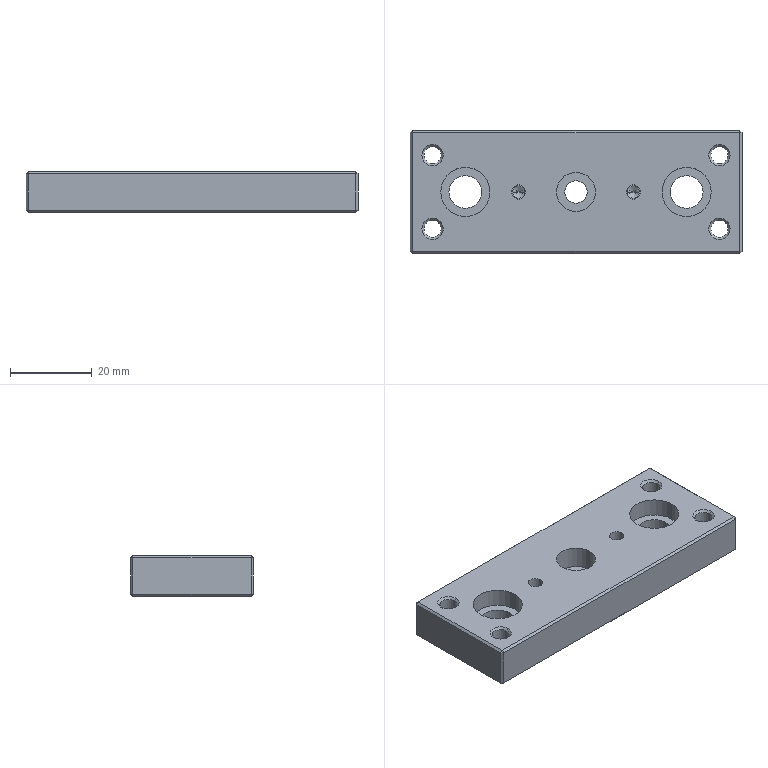Part | 1 solid | 88 faces | box 81 x 30 x 10 mm | volume 21217 mm3 | cylinder 34 | plane 34 | cone 20 | commonest cylinder face diameters 4.2 x8 12 x8 3 x4 3.5 x4 8 x4 5.5 x2